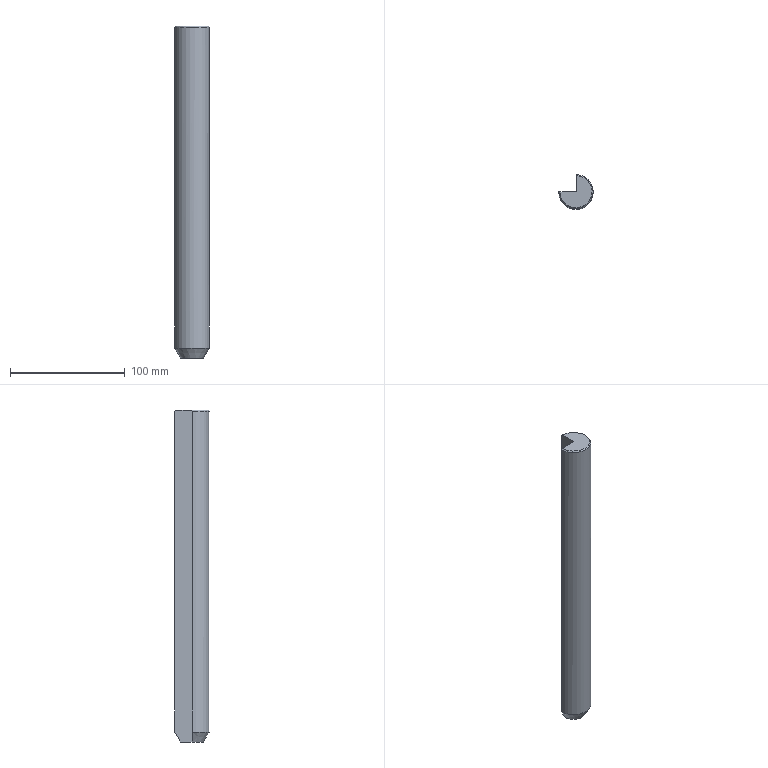Part | STEP file | Clip jig-small post | 1 solid | 26 faces | box 30 x 29.992 x 289.3 mm | volume 149299 mm3 | cylinder 13 | plane 10 | cone 3 | commonest cylinder face diameters 3.3 x12 30 x1